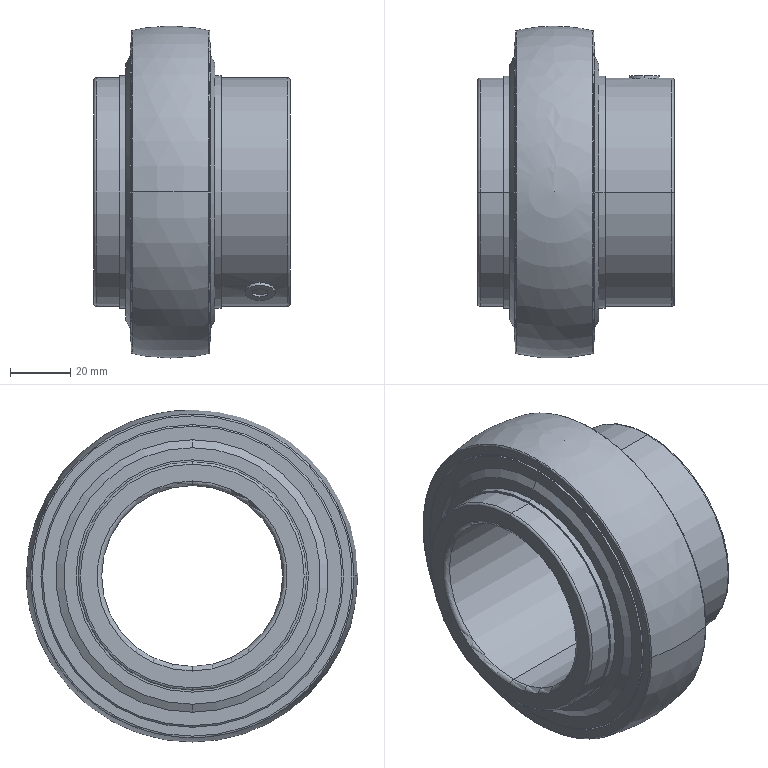Part | SolidWorks | features BaseBody 1 | 1 solid | 184 faces | box 65.1 x 110 x 110 mm | volume 162479 mm3 | cone 60 | cylinder 46 | plane 42 | torus 34 | sphere 2 | commonest cylinder face diameters 75.64 x14 10 x4 76.99 x4 77.154 x4 77.911 x4 97.7 x4